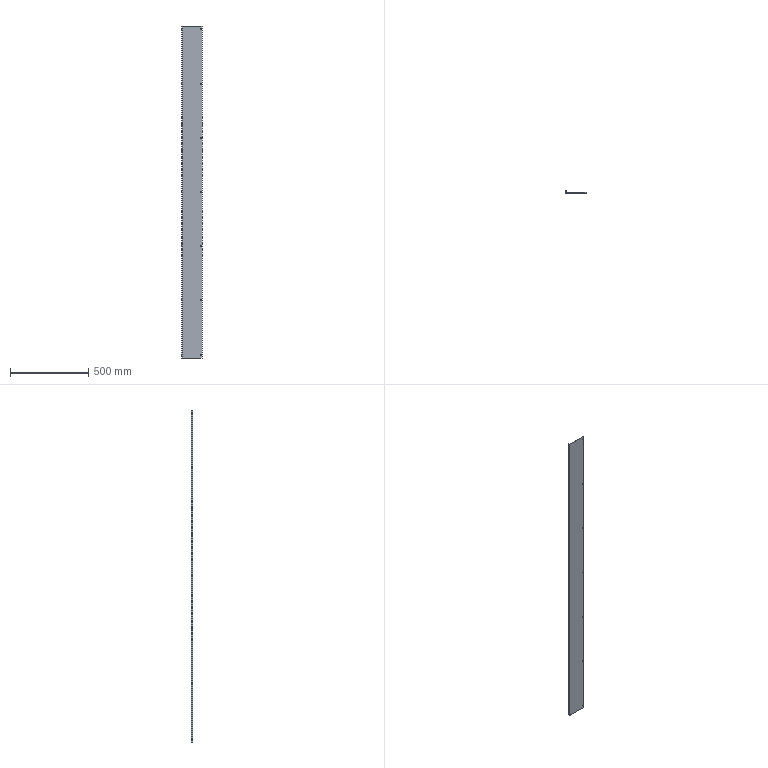Part | SolidWorks | features ICE 4, FlatPattern 1, SMBaseFlange 1, SheetMetal 1 | 1 solid | 77 faces | box 128 x 12 x 2116 mm | volume 293038 mm3 | plane 40 | cylinder 37 | commonest cylinder face diameters 5 x35 0.4 x1 2.4 x1